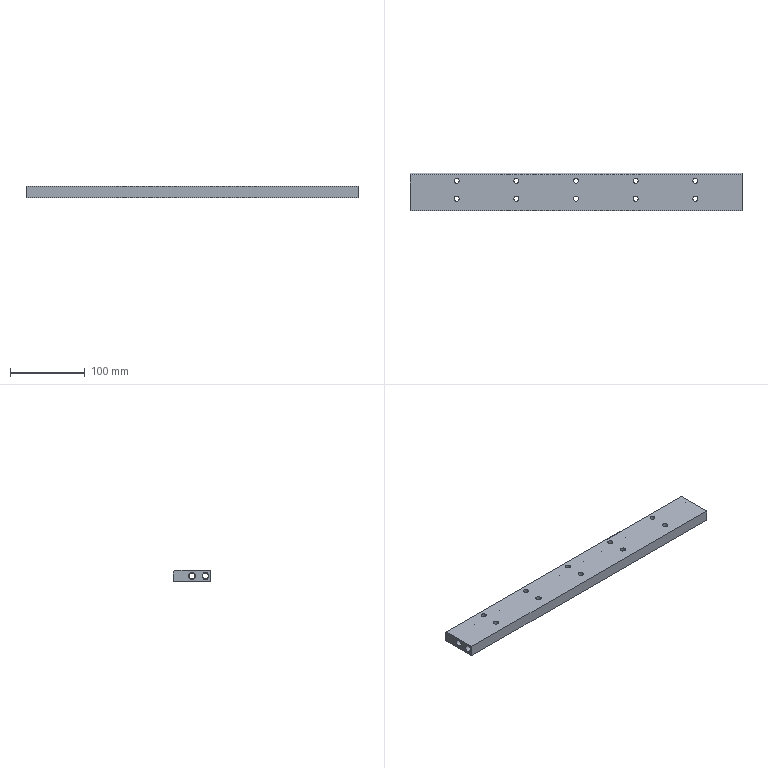Part | STEP file | LM-05-1206 modified_default | 1 solid | 214 faces | box 445 x 50 x 15 mm | volume 275909 mm3 | cylinder 130 | cone 56 | plane 28 | commonest cylinder face diameters 2 x24 4.2 x24 5 x24 6.5 x24 6.6 x10 7 x10